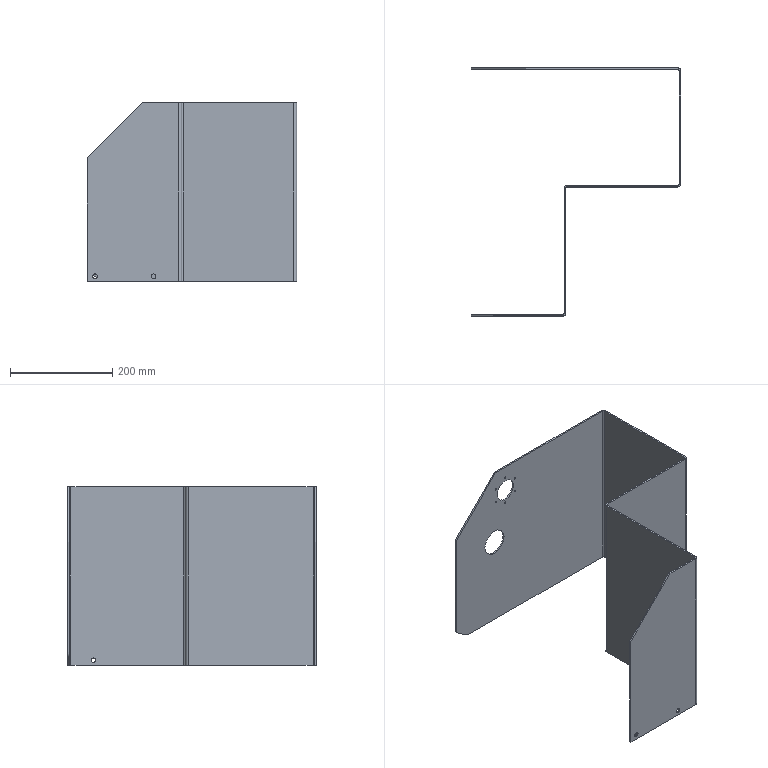Part | SolidWorks | features BaseBody 1 | 1 solid | 65 faces | box 410 x 486 x 350 mm | volume 1308864 mm3 | plane 33 | cylinder 32 | commonest cylinder face diameters 3.3 x12 9 x6 6 x4 12 x4 20 x2 45 x2